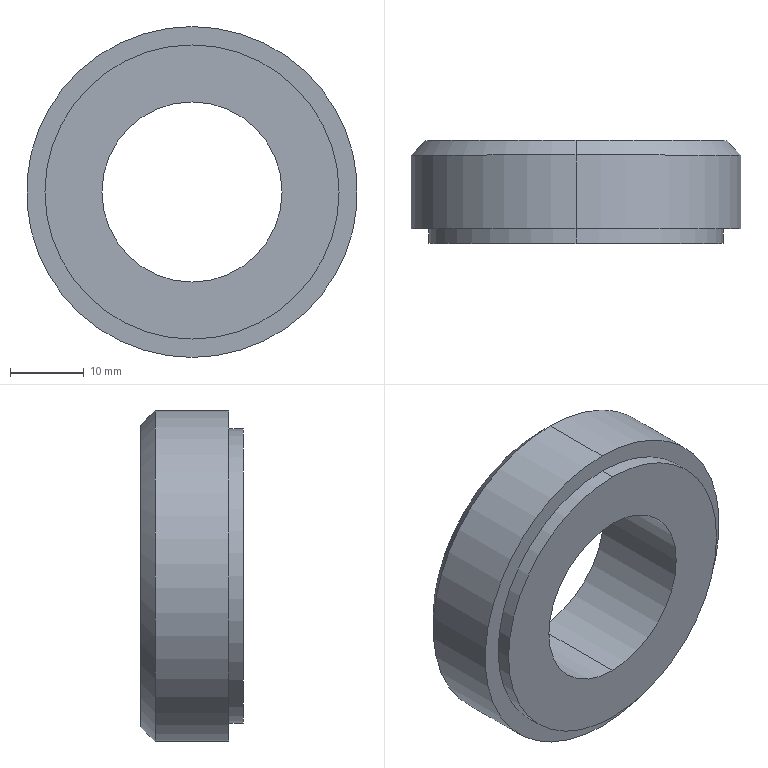Part | SolidWorks | features HoleWzd 1, Revolution 1 | 1 solid | 11 faces | box 45 x 14 x 45 mm | volume 14724 mm3 | cylinder 6 | plane 3 | cone 2 | commonest cylinder face diameters 24.5 x2 40 x2 45 x2
STEP:
#1=CARTESIAN_POINT('',(0.,0.,12.25));
#2=VERTEX_POINT('',#1);
#3=CARTESIAN_POINT('',(0.,0.,-12.25));
#4=VERTEX_POINT('',#3);
#5=CARTESIAN_POINT('',(0.,0.,0.));
#6=DIRECTION('',(0.,-1.,0.));
#7=DIRECTION('',(0.,0.,-1.));
#8=AXIS2_PLACEMENT_3D('',#5,#6,#7);
#9=CIRCLE('',#8,12.25);
#10=EDGE_CURVE('',#2,#4,#9,.T.);
#11=ORIENTED_EDGE('',*,*,#10,.T.);
#12=CARTESIAN_POINT('',(0.,14.,-12.25));
#13=VERTEX_POINT('',#12);
#14=CARTESIAN_POINT('',(0.,14.,-12.25));
#15=DIRECTION('',(0.,1.,0.));
#16=VECTOR('',#15,1000.);
#17=LINE('',#14,#16);
#18=EDGE_CURVE('',#4,#13,#17,.T.);
#19=ORIENTED_EDGE('',*,*,#18,.T.);
#20=CARTESIAN_POINT('',(0.,14.,12.25));
#21=VERTEX_POINT('',#20);
#22=CARTESIAN_POINT('',(0.,14.,0.));
#23=DIRECTION('',(0.,1.,0.));
#24=DIRECTION('',(0.,0.,1.));
#25=AXIS2_PLACEMENT_3D('',#22,#23,#24);
#26=CIRCLE('',#25,12.25);
#27=EDGE_CURVE('',#13,#21,#26,.T.);
#28=ORIENTED_EDGE('',*,*,#27,.T.);
#29=CARTESIAN_POINT('',(0.,14.,12.25));
#30=DIRECTION('',(0.,1.,0.));
#31=VECTOR('',#30,1000.);
#32=LINE('',#29,#31);
#33=EDGE_CURVE('',#2,#21,#32,.T.);
#34=ORIENTED_EDGE('',*,*,#33,.F.);
#35=EDGE_LOOP('',(#11,#19,#28,#34));
#36=FACE_OUTER_BOUND('',#35,.T.);
#37=CARTESIAN_POINT('',(0.,14.,0.));
#38=DIRECTION('',(0.,1.,0.));
#39=DIRECTION('',(0.,0.,1.));
#40=AXIS2_PLACEMENT_3D('',#37,#38,#39);
#41=CYLINDRICAL_SURFACE('',#40,12.25);
#42=ADVANCED_FACE('',(#36),#41,.F.);
#43=CARTESIAN_POINT('',(0.,14.,-20.5));
#44=VERTEX_POINT('',#43);
#45=CARTESIAN_POINT('',(0.,14.,20.5));
#46=VERTEX_POINT('',#45);
#47=CARTESIAN_POINT('',(0.,14.,0.));
#48=DIRECTION('',(0.,-1.,0.));
#49=DIRECTION('',(0.,0.,-1.));
#50=AXIS2_PLACEMENT_3D('',#47,#48,#49);
#51=CIRCLE('',#50,20.5);
#52=EDGE_CURVE('',#44,#46,#51,.T.);
#53=ORIENTED_EDGE('',*,*,#52,.T.);
#54=CARTESIAN_POINT('',(0.,12.,22.5));
#55=VERTEX_POINT('',#54);
#56=CARTESIAN_POINT('',(0.,12.,22.5));
#57=DIRECTION('',(0.,-0.7071,0.7071));
#58=VECTOR('',#57,1000.);
#59=LINE('',#56,#58);
#60=EDGE_CURVE('',#46,#55,#59,.T.);
#61=ORIENTED_EDGE('',*,*,#60,.T.);
#62=CARTESIAN_POINT('',(0.,12.,-22.5));
#63=VERTEX_POINT('',#62);
#64=CARTESIAN_POINT('',(0.,12.,0.));
#65=DIRECTION('',(0.,-1.,0.));
#66=DIRECTION('',(0.,0.,-1.));
#67=AXIS2_PLACEMENT_3D('',#64,#65,#66);
#68=CIRCLE('',#67,22.5);
#69=EDGE_CURVE('',#63,#55,#68,.T.);
#70=ORIENTED_EDGE('',*,*,#69,.F.);
#71=CARTESIAN_POINT('',(0.,12.,-22.5));
#72=DIRECTION('',(0.,-0.7071,-0.7071));
#73=VECTOR('',#72,1000.);
#74=LINE('',#71,#73);
#75=EDGE_CURVE('',#44,#63,#74,.T.);
#76=ORIENTED_EDGE('',*,*,#75,.F.);
#77=EDGE_LOOP('',(#53,#61,#70,#76));
#78=FACE_OUTER_BOUND('',#77,.T.);
#79=CARTESIAN_POINT('',(0.,12.,0.));
#80=DIRECTION('',(0.,-1.,0.));
#81=DIRECTION('',(0.,0.,-1.));
#82=AXIS2_PLACEMENT_3D('',#79,#80,#81);
#83=CONICAL_SURFACE('',#82,22.5,0.7854);
#84=ADVANCED_FACE('',(#78),#83,.T.);
#85=ORIENTED_EDGE('',*,*,#69,.T.);
#86=CARTESIAN_POINT('',(0.,2.,22.5));
#87=VERTEX_POINT('',#86);
#88=CARTESIAN_POINT('',(0.,0.,22.5));
#89=DIRECTION('',(0.,-1.,0.));
#90=VECTOR('',#89,1000.);
#91=LINE('',#88,#90);
#92=EDGE_CURVE('',#55,#87,#91,.T.);
#93=ORIENTED_EDGE('',*,*,#92,.T.);
#94=CARTESIAN_POINT('',(0.,2.,-22.5));
#95=VERTEX_POINT('',#94);
#96=CARTESIAN_POINT('',(0.,2.,0.));
#97=DIRECTION('',(0.,-1.,0.));
#98=DIRECTION('',(0.,0.,-1.));
#99=AXIS2_PLACEMENT_3D('',#96,#97,#98);
#100=CIRCLE('',#99,22.5);
#101=EDGE_CURVE('',#95,#87,#100,.T.);
#102=ORIENTED_EDGE('',*,*,#101,.F.);
#103=CARTESIAN_POINT('',(0.,0.,-22.5));
#104=DIRECTION('',(0.,-1.,0.));
#105=VECTOR('',#104,1000.);
#106=LINE('',#103,#105);
#107=EDGE_CURVE('',#63,#95,#106,.T.);
#108=ORIENTED_EDGE('',*,*,#107,.F.);
#109=EDGE_LOOP('',(#85,#93,#102,#108));
#110=FACE_OUTER_BOUND('',#109,.T.);
#111=CARTESIAN_POINT('',(0.,0.,0.));
#112=DIRECTION('',(0.,-1.,0.));
#113=DIRECTION('',(0.,0.,-1.));
#114=AXIS2_PLACEMENT_3D('',#111,#112,#113);
#115=CYLINDRICAL_SURFACE('',#114,22.5);
#116=ADVANCED_FACE('',(#110),#115,.T.);
#117=CARTESIAN_POINT('',(0.,2.,-20.));
#118=VERTEX_POINT('',#117);
#119=CARTESIAN_POINT('',(0.,2.,20.));
#120=VERTEX_POINT('',#119);
#121=CARTESIAN_POINT('',(0.,2.,0.));
#122=DIRECTION('',(0.,-1.,0.));
#123=DIRECTION('',(0.,0.,-1.));
#124=AXIS2_PLACEMENT_3D('',#121,#122,#123);
#125=CIRCLE('',#124,20.);
#126=EDGE_CURVE('',#118,#120,#125,.T.);
#127=ORIENTED_EDGE('',*,*,#126,.T.);
#128=CARTESIAN_POINT('',(0.,0.,20.));
#129=VERTEX_POINT('',#128);
#130=CARTESIAN_POINT('',(0.,0.,20.));
#131=DIRECTION('',(0.,-1.,0.));
#132=VECTOR('',#131,1000.);
#133=LINE('',#130,#132);
#134=EDGE_CURVE('',#120,#129,#133,.T.);
#135=ORIENTED_EDGE('',*,*,#134,.T.);
#136=CARTESIAN_POINT('',(0.,0.,-20.));
#137=VERTEX_POINT('',#136);
#138=CARTESIAN_POINT('',(0.,0.,0.));
#139=DIRECTION('',(0.,-1.,0.));
#140=DIRECTION('',(0.,0.,-1.));
#141=AXIS2_PLACEMENT_3D('',#138,#139,#140);
#142=CIRCLE('',#141,20.);
#143=EDGE_CURVE('',#137,#129,#142,.T.);
#144=ORIENTED_EDGE('',*,*,#143,.F.);
#145=CARTESIAN_POINT('',(0.,0.,-20.));
#146=DIRECTION('',(0.,-1.,0.));
#147=VECTOR('',#146,1000.);
#148=LINE('',#145,#147);
#149=EDGE_CURVE('',#118,#137,#148,.T.);
#150=ORIENTED_EDGE('',*,*,#149,.F.);
#151=EDGE_LOOP('',(#127,#135,#144,#150));
#152=FACE_OUTER_BOUND('',#151,.T.);
#153=CARTESIAN_POINT('',(0.,0.,0.));
#154=DIRECTION('',(0.,-1.,0.));
#155=DIRECTION('',(0.,0.,-1.));
#156=AXIS2_PLACEMENT_3D('',#153,#154,#155);
#157=CYLINDRICAL_SURFACE('',#156,20.);
#158=ADVANCED_FACE('',(#152),#157,.T.);
#159=ORIENTED_EDGE('',*,*,#10,.F.);
#160=CARTESIAN_POINT('',(0.,0.,0.));
#161=DIRECTION('',(0.,-1.,0.));
#162=DIRECTION('',(0.,0.,-1.));
#163=AXIS2_PLACEMENT_3D('',#160,#161,#162);
#164=CIRCLE('',#163,12.25);
#165=EDGE_CURVE('',#4,#2,#164,.T.);
#166=ORIENTED_EDGE('',*,*,#165,.F.);
#167=EDGE_LOOP('',(#159,#166));
#168=FACE_BOUND('',#167,.T.);
#169=ORIENTED_EDGE('',*,*,#143,.T.);
#170=CARTESIAN_POINT('',(0.,0.,0.));
#171=DIRECTION('',(0.,-1.,0.));
#172=DIRECTION('',(0.,0.,-1.));
#173=AXIS2_PLACEMENT_3D('',#170,#171,#172);
#174=CIRCLE('',#173,20.);
#175=EDGE_CURVE('',#129,#137,#174,.T.);
#176=ORIENTED_EDGE('',*,*,#175,.T.);
#177=EDGE_LOOP('',(#169,#176));
#178=FACE_OUTER_BOUND('',#177,.T.);
#179=CARTESIAN_POINT('',(0.,0.,-12.));
#180=DIRECTION('',(0.,-1.,0.));
#181=DIRECTION('',(0.,0.,-1.));
#182=AXIS2_PLACEMENT_3D('',#179,#180,#181);
#183=PLANE('',#182);
#184=ADVANCED_FACE('',(#168,#178),#183,.T.);
#185=ORIENTED_EDGE('',*,*,#134,.F.);
#186=CARTESIAN_POINT('',(0.,2.,0.));
#187=DIRECTION('',(0.,-1.,0.));
#188=DIRECTION('',(0.,0.,-1.));
#189=AXIS2_PLACEMENT_3D('',#186,#187,#188);
#190=CIRCLE('',#189,20.);
#191=EDGE_CURVE('',#120,#118,#190,.T.);
#192=ORIENTED_EDGE('',*,*,#191,.T.);
#193=ORIENTED_EDGE('',*,*,#149,.T.);
#194=ORIENTED_EDGE('',*,*,#175,.F.);
#195=EDGE_LOOP('',(#185,#192,#193,#194));
#196=FACE_OUTER_BOUND('',#195,.T.);
#197=CARTESIAN_POINT('',(0.,0.,0.));
#198=DIRECTION('',(0.,-1.,0.));
#199=DIRECTION('',(0.,0.,-1.));
#200=AXIS2_PLACEMENT_3D('',#197,#198,#199);
#201=CYLINDRICAL_SURFACE('',#200,20.);
#202=ADVANCED_FACE('',(#196),#201,.T.);
#203=ORIENTED_EDGE('',*,*,#101,.T.);
#204=CARTESIAN_POINT('',(0.,2.,0.));
#205=DIRECTION('',(0.,-1.,0.));
#206=DIRECTION('',(0.,0.,-1.));
#207=AXIS2_PLACEMENT_3D('',#204,#205,#206);
#208=CIRCLE('',#207,22.5);
#209=EDGE_CURVE('',#87,#95,#208,.T.);
#210=ORIENTED_EDGE('',*,*,#209,.T.);
#211=EDGE_LOOP('',(#203,#210));
#212=FACE_OUTER_BOUND('',#211,.T.);
#213=ORIENTED_EDGE('',*,*,#126,.F.);
#214=ORIENTED_EDGE('',*,*,#191,.F.);
#215=EDGE_LOOP('',(#213,#214));
#216=FACE_BOUND('',#215,.T.);
#217=CARTESIAN_POINT('',(0.,2.,-20.));
#218=DIRECTION('',(0.,-1.,0.));
#219=DIRECTION('',(0.,0.,-1.));
#220=AXIS2_PLACEMENT_3D('',#217,#218,#219);
#221=PLANE('',#220);
#222=ADVANCED_FACE('',(#212,#216),#221,.T.);
#223=ORIENTED_EDGE('',*,*,#92,.F.);
#224=CARTESIAN_POINT('',(0.,12.,0.));
#225=DIRECTION('',(0.,-1.,0.));
#226=DIRECTION('',(0.,0.,-1.));
#227=AXIS2_PLACEMENT_3D('',#224,#225,#226);
#228=CIRCLE('',#227,22.5);
#229=EDGE_CURVE('',#55,#63,#228,.T.);
#230=ORIENTED_EDGE('',*,*,#229,.T.);
#231=ORIENTED_EDGE('',*,*,#107,.T.);
#232=ORIENTED_EDGE('',*,*,#209,.F.);
#233=EDGE_LOOP('',(#223,#230,#231,#232));
#234=FACE_OUTER_BOUND('',#233,.T.);
#235=CARTESIAN_POINT('',(0.,0.,0.));
#236=DIRECTION('',(0.,-1.,0.));
#237=DIRECTION('',(0.,0.,-1.));
#238=AXIS2_PLACEMENT_3D('',#235,#236,#237);
#239=CYLINDRICAL_SURFACE('',#238,22.5);
#240=ADVANCED_FACE('',(#234),#239,.T.);
#241=ORIENTED_EDGE('',*,*,#60,.F.);
#242=CARTESIAN_POINT('',(0.,14.,0.));
#243=DIRECTION('',(0.,-1.,0.));
#244=DIRECTION('',(0.,0.,-1.));
#245=AXIS2_PLACEMENT_3D('',#242,#243,#244);
#246=CIRCLE('',#245,20.5);
#247=EDGE_CURVE('',#46,#44,#246,.T.);
#248=ORIENTED_EDGE('',*,*,#247,.T.);
#249=ORIENTED_EDGE('',*,*,#75,.T.);
#250=ORIENTED_EDGE('',*,*,#229,.F.);
#251=EDGE_LOOP('',(#241,#248,#249,#250));
#252=FACE_OUTER_BOUND('',#251,.T.);
#253=CARTESIAN_POINT('',(0.,12.,0.));
#254=DIRECTION('',(0.,-1.,0.));
#255=DIRECTION('',(0.,0.,-1.));
#256=AXIS2_PLACEMENT_3D('',#253,#254,#255);
#257=CONICAL_SURFACE('',#256,22.5,0.7854);
#258=ADVANCED_FACE('',(#252),#257,.T.);
#259=CARTESIAN_POINT('',(0.,14.,0.));
#260=DIRECTION('',(0.,1.,0.));
#261=DIRECTION('',(0.,0.,1.));
#262=AXIS2_PLACEMENT_3D('',#259,#260,#261);
#263=CIRCLE('',#262,12.25);
#264=EDGE_CURVE('',#21,#13,#263,.T.);
#265=ORIENTED_EDGE('',*,*,#264,.F.);
#266=ORIENTED_EDGE('',*,*,#27,.F.);
#267=EDGE_LOOP('',(#265,#266));
#268=FACE_BOUND('',#267,.T.);
#269=ORIENTED_EDGE('',*,*,#52,.F.);
#270=ORIENTED_EDGE('',*,*,#247,.F.);
#271=EDGE_LOOP('',(#269,#270));
#272=FACE_OUTER_BOUND('',#271,.T.);
#273=CARTESIAN_POINT('',(0.,14.,-20.5));
#274=DIRECTION('',(0.,1.,0.));
#275=DIRECTION('',(0.,0.,1.));
#276=AXIS2_PLACEMENT_3D('',#273,#274,#275);
#277=PLANE('',#276);
#278=ADVANCED_FACE('',(#268,#272),#277,.T.);
#279=ORIENTED_EDGE('',*,*,#18,.F.);
#280=ORIENTED_EDGE('',*,*,#165,.T.);
#281=ORIENTED_EDGE('',*,*,#33,.T.);
#282=ORIENTED_EDGE('',*,*,#264,.T.);
#283=EDGE_LOOP('',(#279,#280,#281,#282));
#284=FACE_OUTER_BOUND('',#283,.T.);
#285=CARTESIAN_POINT('',(0.,14.,0.));
#286=DIRECTION('',(0.,1.,0.));
#287=DIRECTION('',(0.,0.,1.));
#288=AXIS2_PLACEMENT_3D('',#285,#286,#287);
#289=CYLINDRICAL_SURFACE('',#288,12.25);
#290=ADVANCED_FACE('',(#284),#289,.F.);
#291=CLOSED_SHELL('',(#42,#84,#116,#158,#184,#202,#222,#240,#258,#278,#290));
#292=MANIFOLD_SOLID_BREP('',#291);
#293=CARTESIAN_POINT('',(0.,0.,0.));
#294=DIRECTION('',(0.,0.,1.));
#295=DIRECTION('',(1.,0.,0.));
#296=AXIS2_PLACEMENT_3D('',#293,#294,#295);
#297=(LENGTH_UNIT()NAMED_UNIT(*)SI_UNIT(.MILLI.,.METRE.));
#298=UNCERTAINTY_MEASURE_WITH_UNIT(LENGTH_MEASURE(0.00001),#297,'','');
#299=(NAMED_UNIT(*)PLANE_ANGLE_UNIT()SI_UNIT($,.RADIAN.));
#300=(NAMED_UNIT(*)SI_UNIT($,.STERADIAN.)SOLID_ANGLE_UNIT());
#301=(GEOMETRIC_REPRESENTATION_CONTEXT(3)GLOBAL_UNCERTAINTY_ASSIGNED_CONTEXT((#298))GLOBAL_UNIT_ASSIGNED_CONTEXT((#297,#299,#300))REPRESENTATION_CONTEXT('',''));
#302=ADVANCED_BREP_SHAPE_REPRESENTATION('',(#292,#296),#301);